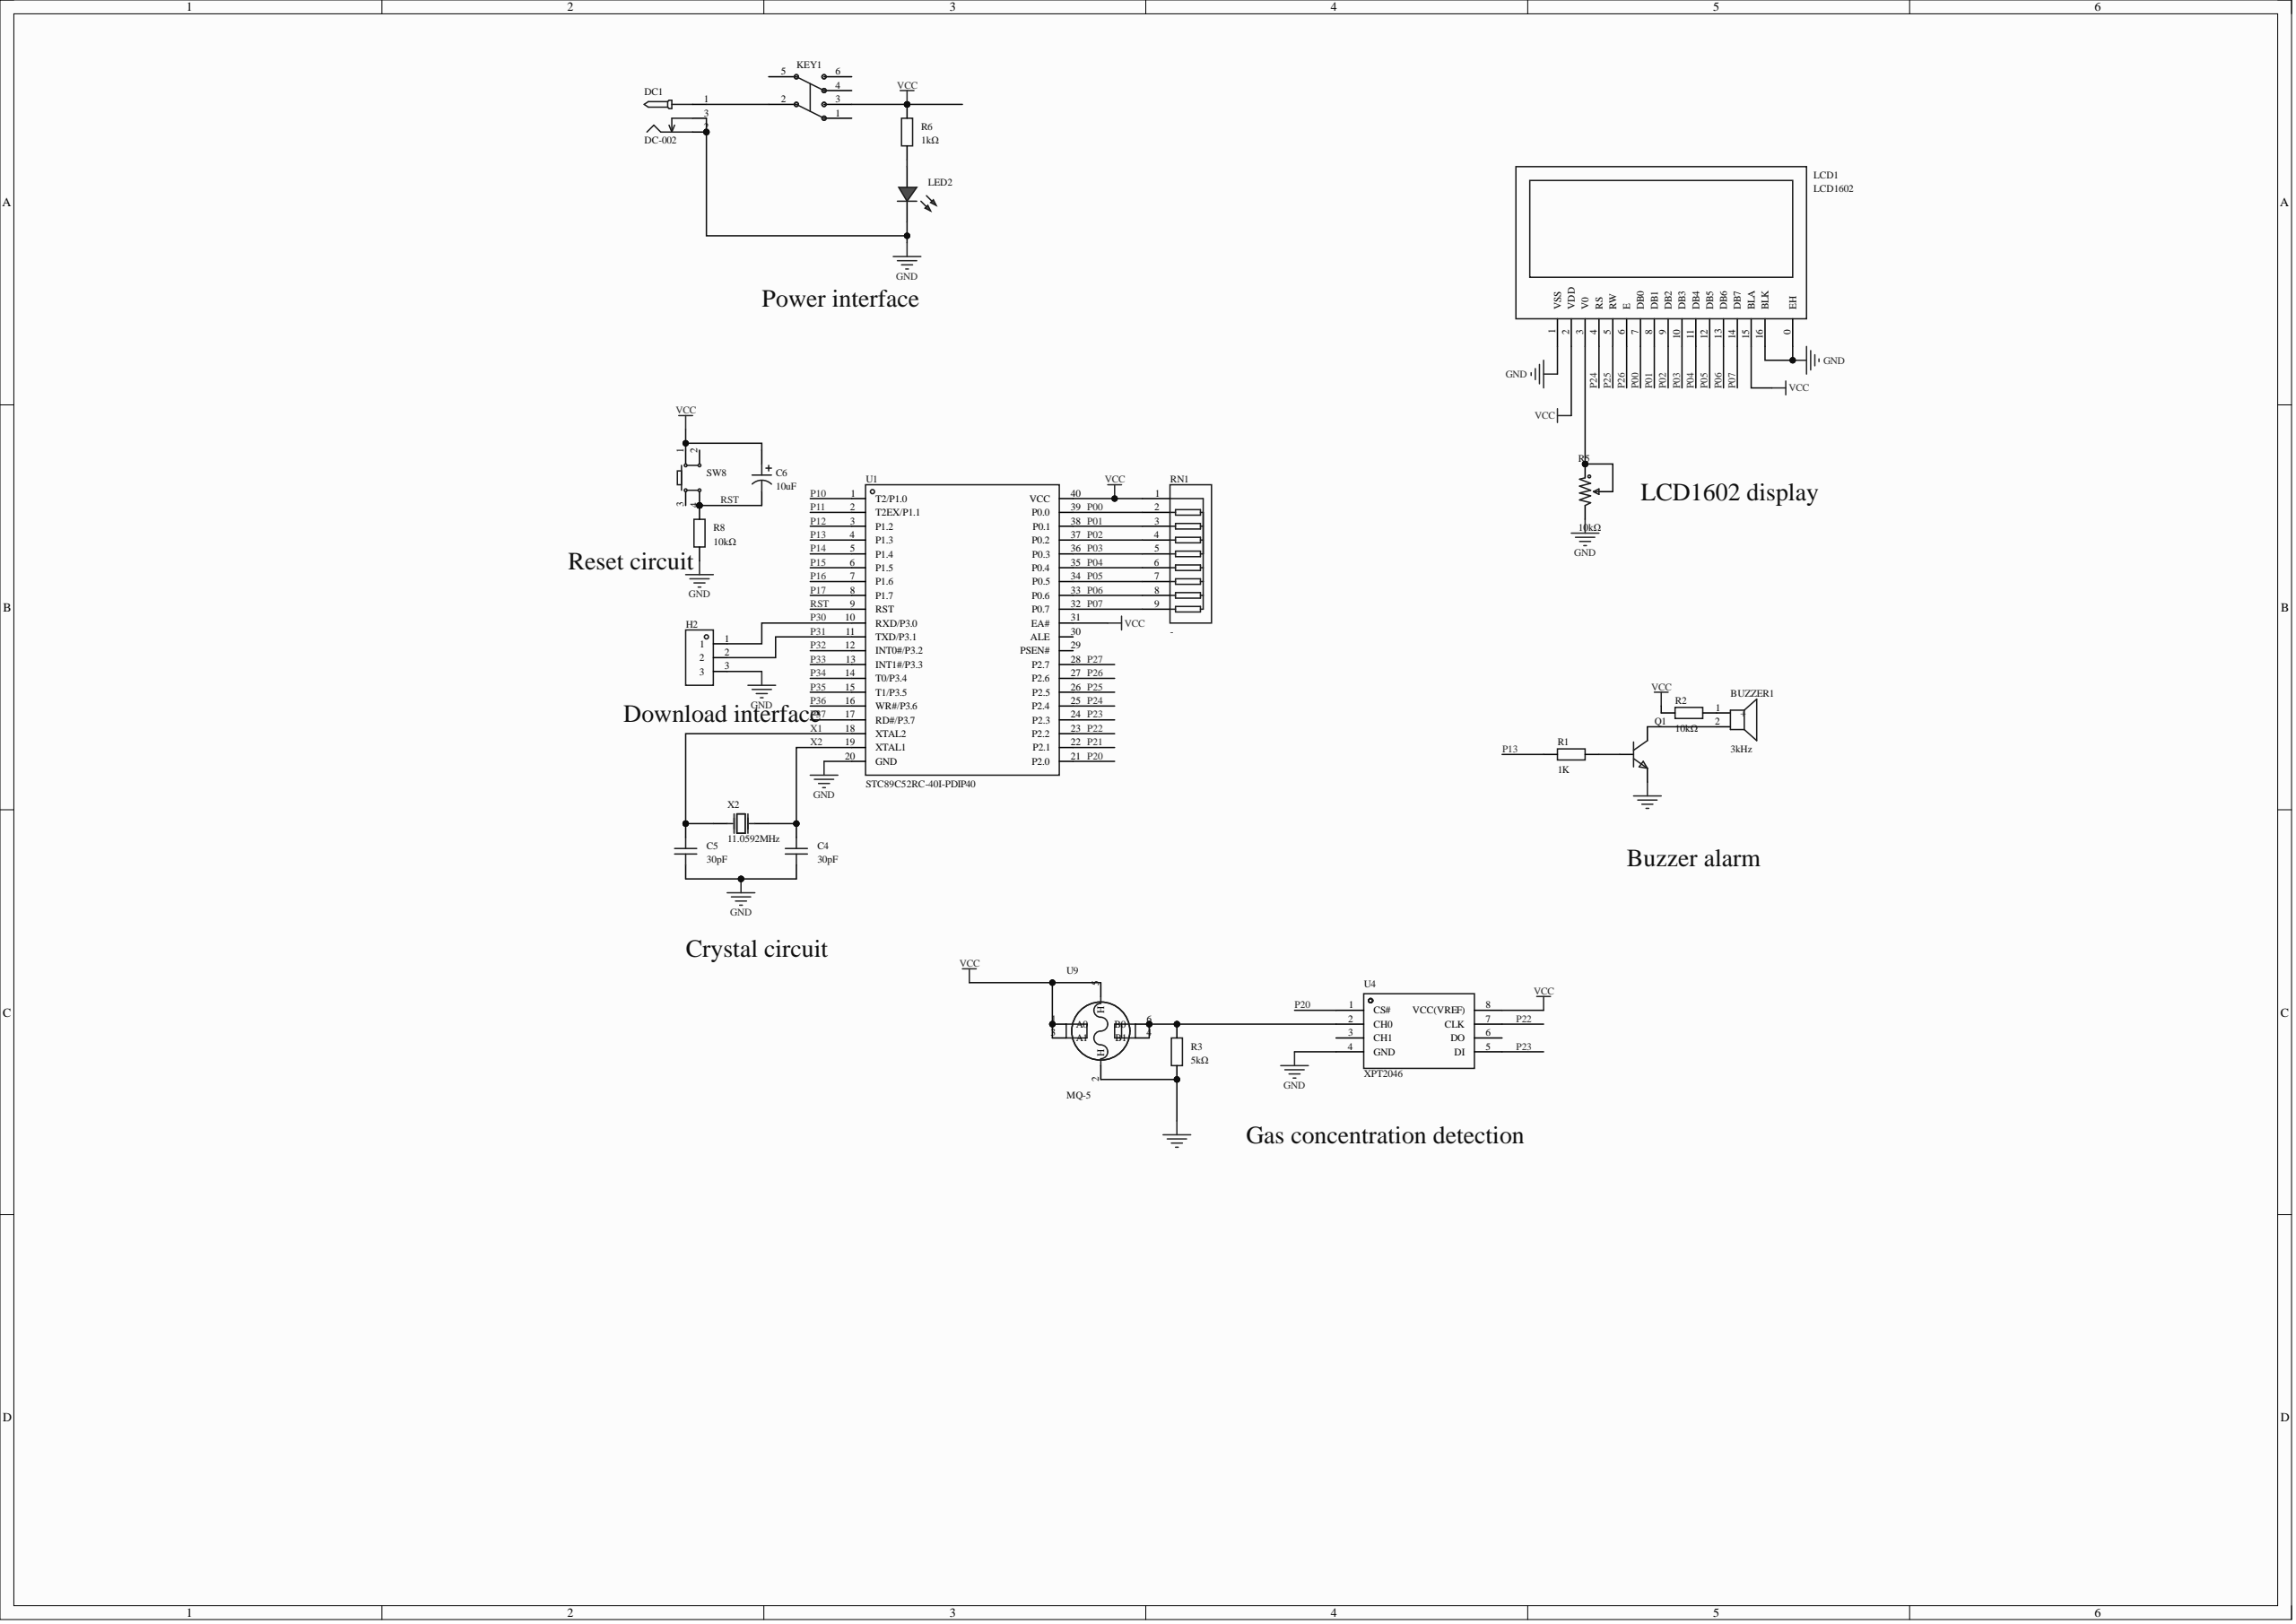Circuit board | Altium Designer | 22 parts | 29 nets
Bill of materials:
Comment,Description,Designator,Footprint,LibRef,Quantity
"3kHz","Drive mode: active (built-in driver circuit); construction type: electromagnetic; frequency: 3kHz; sound pressure (SPL): 85dB;","BUZZER1","BUZ-TH_BD9.6-P5.00-D0.7-FD","HNB09A05","1"
"30pF","Capacitance: 30pF; tolerance: ±10%; rated voltage: 25V; temperature coefficient: C0G;","C4, C5","CAP-TH_L3.8-W2.5-P2.54-D0.50","C315C300K3G5TA7301","2"
"10uF","Capacitance: 10uF; tolerance: ±20%; rated voltage: 50V; ripple current: 120mA@100KHz; equivalent series resistance (ESR): 1.6Ω;","C6","CAP-TH_BD5.0-P2.00-D0.8-FD-10UF50VC110GL","10UF50VC110GL","1"
"DC-002","","DC1","DC-IN-TH_DC-3510","DC-002","1"
"","","H2","HDR-TH_3P-P2.54-V-M","HDR-M_2.54_1x3P","1"
"Non-latching switch 8.5×8.5 silent","6 pins, 8.5×8.5","KEY1","SW-TH_6P-L8.5-W8.5-P2.54","无自锁开关 8.5×8.5 无声","1"
"LCD1602","Controller IC: SPLC780; size (inch): 2;","LCD1","LCD1602","HS1602A","1"
"","","LED2","LED_TH-3mm","LED_TH-R_3mm","1"
"","","Q1","S8050_TO_92","S8050_TO_NPN","1"
"1K","","R1","Res_1/8W","Res_AXIAL-1/8W","1"
"10kΩ","","R2, R8","Res_1/8W","Res_AXIAL-1/8W","2"
"5kΩ","","R3","Res_1/8W","Res_AXIAL-1/8W","1"
"10kΩ","Resistance: 10kΩ; tolerance: ±25%; power: 100mW;","R5","RES-ADJ-SMD_RM065-V1","RM065-103(10K)","1"
"1kΩ","","R6","Res_1/8W","Res_AXIAL-1/8W","1"
"-","Number of resistors: -; resistance: -; power per element: -;","RN1","RES-ARRAY-TH_9P-P2.54-D1.0","排阻 10 K 5%","1"
"","","SW8","SW-TH_4P-L6.0-W6.0-P4.50-LS6.5","Key_TH_6x6x6","1"
"STC89C52RC-40I-PDIP40","CPU core: 51 family; CPU max frequency: -;","U1","DIP-40_L52.0-W13.7-P2.54-LS15.2-BL","STC89C52RC-40I-PDIP40","1"
"XPT2046","","U4","DIP-8_L9.7-W6.4-P2.54-LS7.6-BL","ADC0832CCN","1"
"MQ-5","MQ-5 combustible gas sensor, high sensitivity to butane, propane and methane","U9","SENSOR-TH_MQ-5","MQ-5","1"
"11.059MHz","Crystal type: through-hole crystal; frequency: 11.059MHz; room-temperature frequency tolerance: ±20ppm; load capacitance: 30pF;","X2","OSC-TH_L11.1-W4.7-P4.88","9AC11059302060C3","1"
Netlist (Protel format):
[
BUZZER1
BUZ-TH_BD9.6-P5.00-D0.7-FD
3kHz



]
[
C4
CAP-TH_L3.8-W2.5-P2.54-D0.50
30pF



]
[
C5
CAP-TH_L3.8-W2.5-P2.54-D0.50
30pF



]
[
C6
CAP-TH_BD5.0-P2.00-D0.8-FD-10UF50VC110GL
10uF



]
[
DC1
DC-IN-TH_DC-3510
DC-002



]
[
H2
HDR-TH_3P-P2.54-V-M




]
[
KEY1
SW-TH_6P-L8.5-W8.5-P2.54
Non-latching switch 8.5×8.5 silent



]
[
LCD1
LCD1602
LCD1602



]
[
LED2
LED_TH-3mm




]
[
Q1
S8050_TO_92




]
[
R1
Res_1/8W
1K



]
[
R2
Res_1/8W
10kΩ



]
[
R3
Res_1/8W
5kΩ



]
[
R5
RES-ADJ-SMD_RM065-V1
10kΩ



]
[
R6
Res_1/8W
1kΩ



]
[
R8
Res_1/8W
10kΩ



]
[
RN1
RES-ARRAY-TH_9P-P2.54-D1.0
-



]
[
SW8
SW-TH_4P-L6.0-W6.0-P4.50-LS6.5




]
[
U1
DIP-40_L52.0-W13.7-P2.54-LS15.2-BL
STC89C52RC-40I-PDIP40



]
[
U4
DIP-8_L9.7-W6.4-P2.54-LS7.6-BL
XPT2046



]
[
U9
SENSOR-TH_MQ-5
MQ-5



]
[
X2
OSC-TH_L11.1-W4.7-P4.88
11.0592MHz



]
(
X2
C4-2
U1-19
X2-2
)
(
X1
C5-2
U1-18
X2-1
)
(
VCC
C6-1
KEY1-3
LCD1-2
LCD1-15
R2-1
R6-2
RN1-1
SW8-1
U1-31
U1-40
U4-8
U9-1
U9-3
U9-5
)
(
RST
C6-2
R8-2
SW8-4
U1-9
)
(
P31
H2-2
U1-11
)
(
P30
H2-1
U1-10
)
(
P26
LCD1-6
U1-27
)
(
P25
LCD1-5
U1-26
)
(
P24
LCD1-4
U1-25
)
(
P23
U1-24
U4-5
)
(
P22
U1-23
U4-7
)
(
P20
U1-21
U4-1
)
(
P13
R1-1
U1-4
)
(
P07
LCD1-14
RN1-9
U1-32
)
(
P06
LCD1-13
RN1-8
U1-33
)
(
P05
LCD1-12
RN1-7
U1-34
)
(
P04
LCD1-11
RN1-6
U1-35
)
(
P03
LCD1-10
RN1-5
U1-36
)
(
P02
LCD1-9
RN1-4
U1-37
)
(
P01
LCD1-8
RN1-3
U1-38
)
(
P00
LCD1-7
RN1-2
U1-39
)
(
NetR3_2
R3-2
U4-2
U9-4
U9-6
)
(
NetQ1_2
Q1-2
R1-2
)
(
NetLED2_1
LED2-1
R6-1
)
(
NetLCD1_3
LCD1-3
R5-1
R5-2
)
(
NetDC1_1
DC1-1
KEY1-2
)
(
NetBUZZER1_2
BUZZER1-2
Q1-3
)
(
NetBUZZER1_1
BUZZER1-1
R2-2
)
(
GND
C4-1
C5-1
DC1-2
DC1-3
H2-3
LCD1-0
LCD1-1
LCD1-16
LED2-2
Q1-1
R3-1
R5-3
R8-1
U1-20
U4-4
U9-2
)